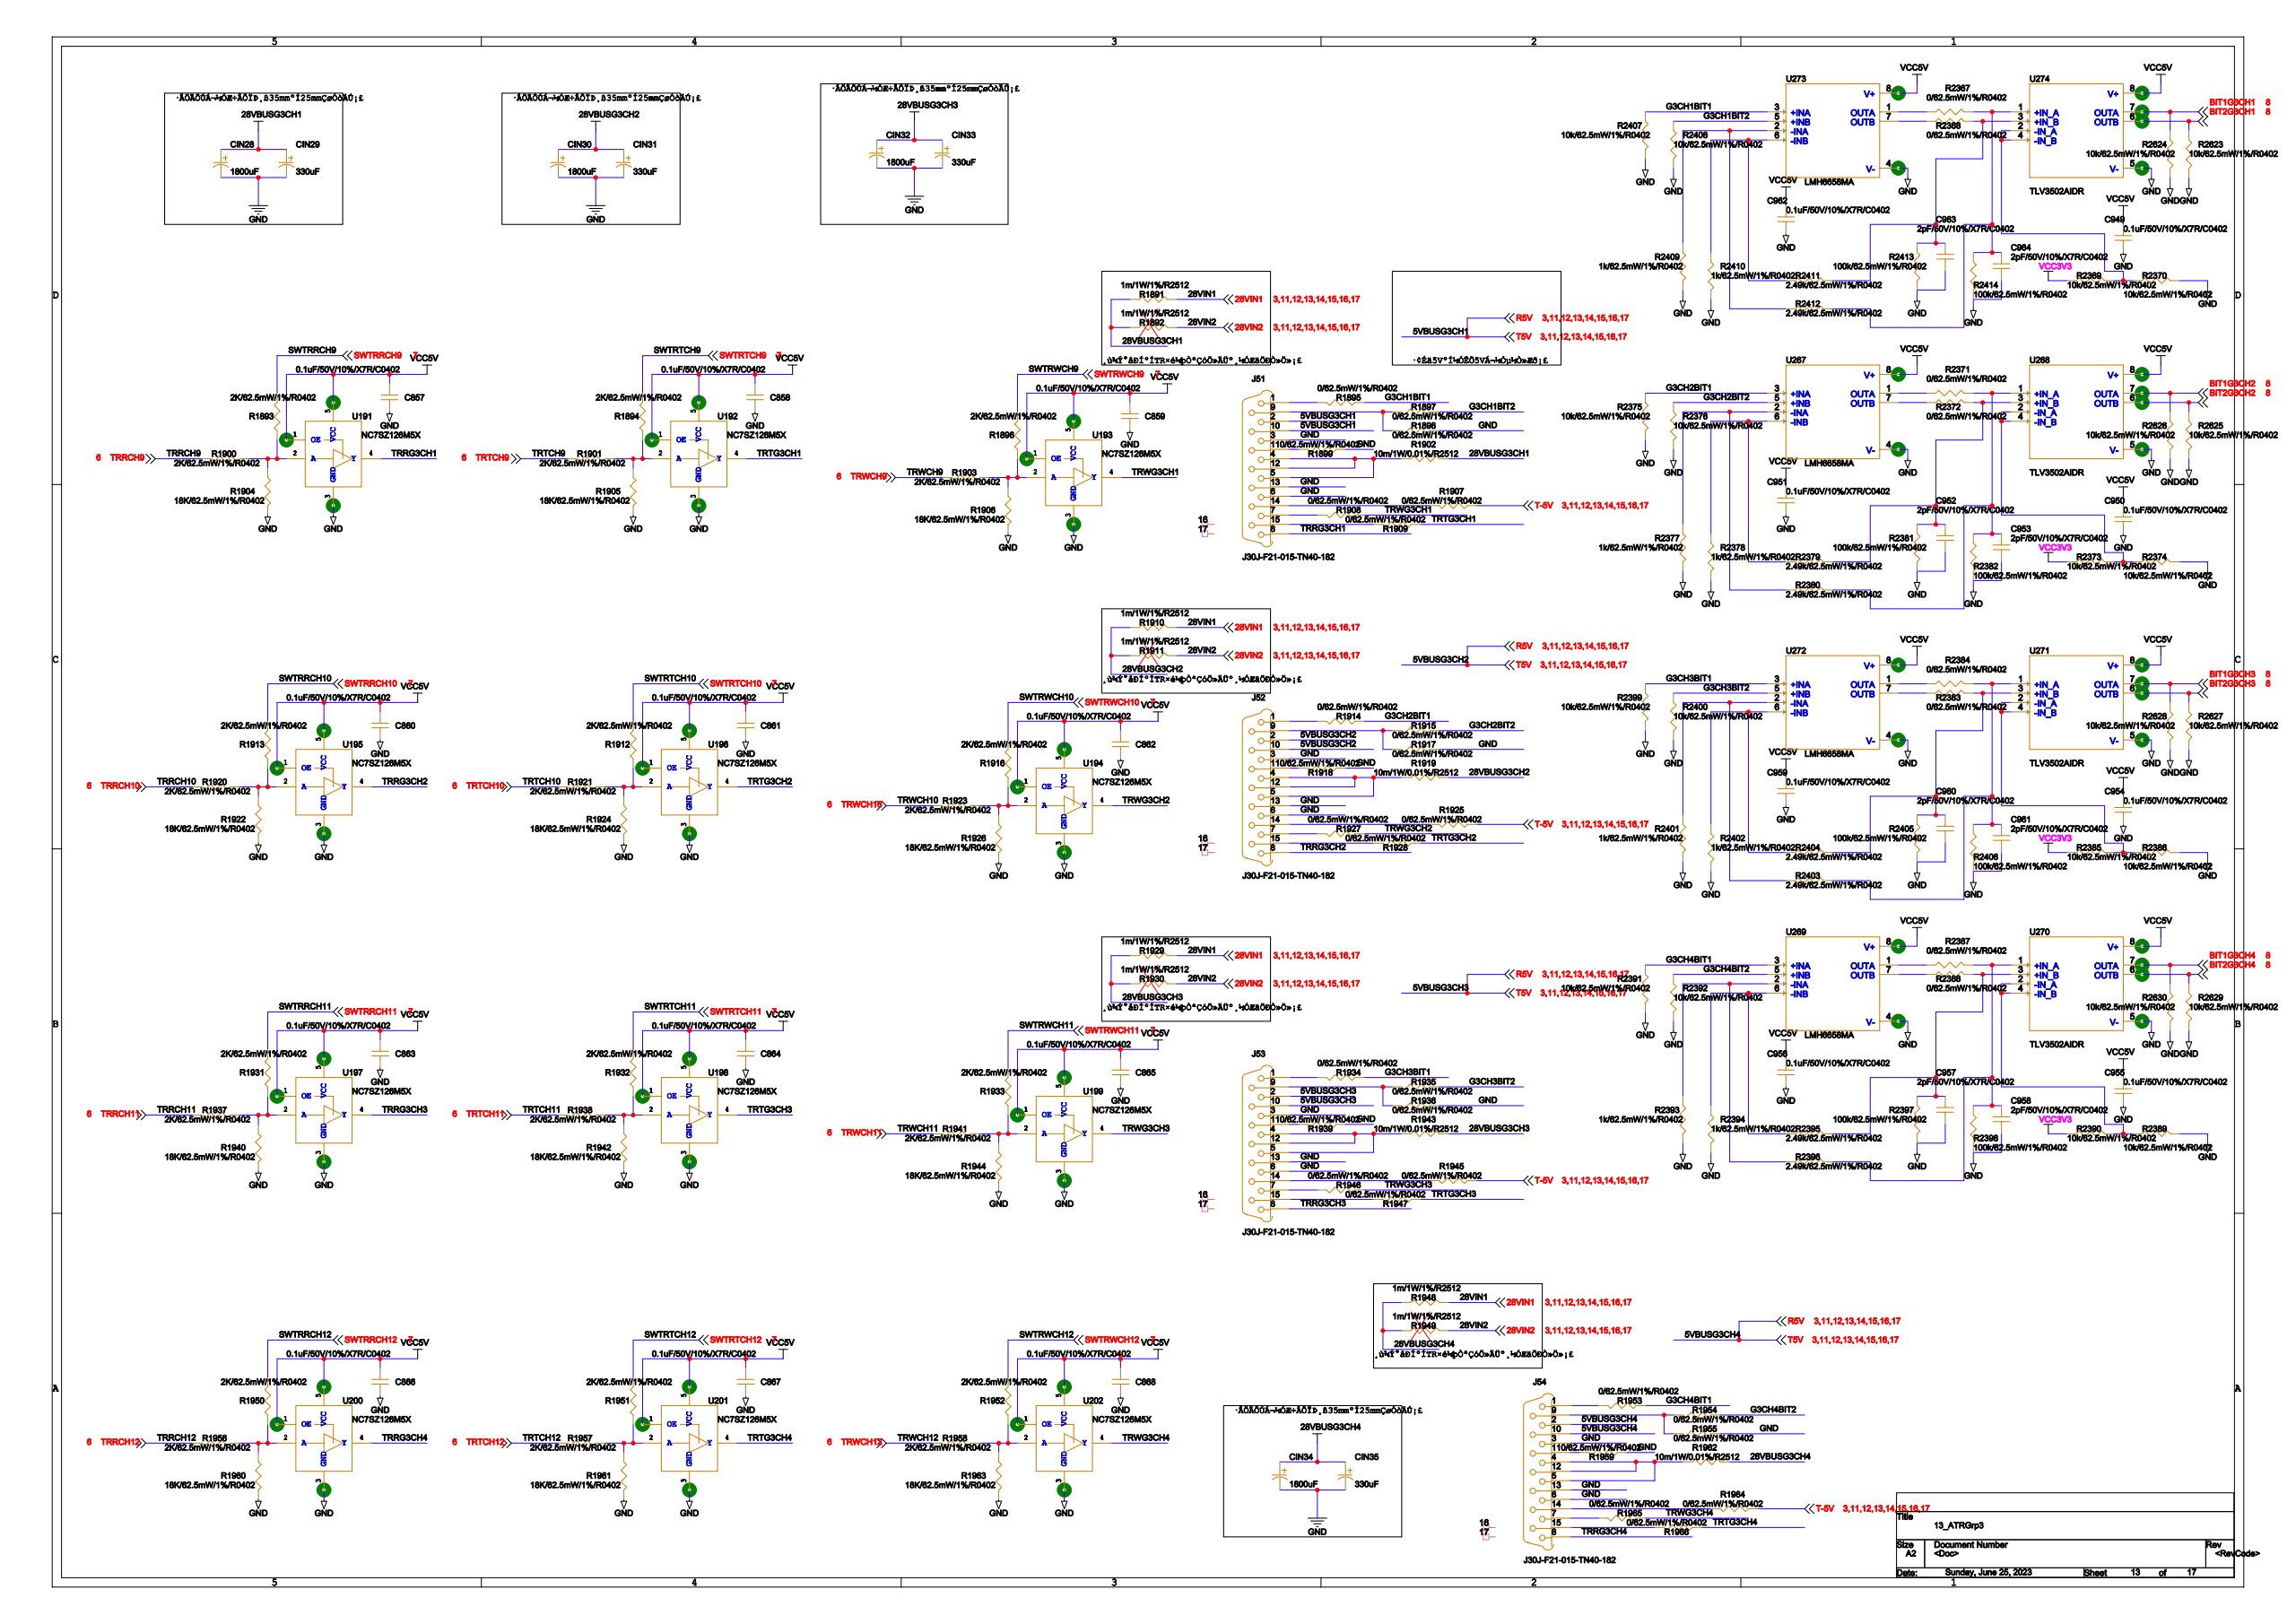Circuit board | Cadence Allegro | 2002 parts | 1538 nets | one sheet of the schematic
Parts on this sheet (reference | value | footprint):
C857 | 0.1uF/50V/10%/X7R/C0402 | 0402
C858 | 0.1uF/50V/10%/X7R/C0402 | 0402
C859 | 0.1uF/50V/10%/X7R/C0402 | 0402
C860 | 0.1uF/50V/10%/X7R/C0402 | 0402
C861 | 0.1uF/50V/10%/X7R/C0402 | 0402
C862 | 0.1uF/50V/10%/X7R/C0402 | 0402
C863 | 0.1uF/50V/10%/X7R/C0402 | 0402
C864 | 0.1uF/50V/10%/X7R/C0402 | 0402
C865 | 0.1uF/50V/10%/X7R/C0402 | 0402
C866 | 0.1uF/50V/10%/X7R/C0402 | 0402
C867 | 0.1uF/50V/10%/X7R/C0402 | 0402
C868 | 0.1uF/50V/10%/X7R/C0402 | 0402
C949 | 0.1uF/50V/10%/X7R/C0402 | 0402
C950 | 0.1uF/50V/10%/X7R/C0402 | 0402
C952 | 2pF/50V/10%/X7R/C0402 | 0402
C953 | 2pF/50V/10%/X7R/C0402 | 0402
C954 | 0.1uF/50V/10%/X7R/C0402 | 0402
C955 | 0.1uF/50V/10%/X7R/C0402 | 0402
C957 | 2pF/50V/10%/X7R/C0402 | 0402
C958 | 2pF/50V/10%/X7R/C0402 | 0402
C960 | 2pF/50V/10%/X7R/C0402 | 0402
C961 | 2pF/50V/10%/X7R/C0402 | 0402
C963 | 2pF/50V/10%/X7R/C0402 | 0402
C964 | 2pF/50V/10%/X7R/C0402 | 0402
CIN28 | ECF1HM182M27OTPO | AP-SMD_BD18-L27-W6_6-LS7_21
CIN29 | ECF1JM331G20OTPO | AP-SMD_BD10-L20-W6_6-LS7_21
CIN30 | ECF1HM182M27OTPO | AP-SMD_BD18-L27-W6_6-LS7_21
CIN31 | ECF1JM331G20OTPO | AP-SMD_BD10-L20-W6_6-LS7_21
CIN32 | ECF1HM182M27OTPO | AP-SMD_BD18-L27-W6_6-LS7_21
CIN33 | ECF1JM331G20OTPO | AP-SMD_BD10-L20-W6_6-LS7_21
CIN34 | ECF1HM182M27OTPO | AP-SMD_BD18-L27-W6_6-LS7_21
CIN35 | ECF1JM331G20OTPO | AP-SMD_BD10-L20-W6_6-LS7_21
J51 | J30J-F21-015-TN40-182 | J30J-F21-015-TN40-182
J52 | J30J-F21-015-TN40-182 | J30J-F21-015-TN40-182
J53 | J30J-F21-015-TN40-182 | J30J-F21-015-TN40-182
J54 | J30J-F21-015-TN40-182 | J30J-F21-015-TN40-182
R1891 | 1m/1W/1%/R2512 | 2512
R1892 | 1m/1W/1%/R2512 | 2512
R1893 | 2K/62.5mW/1%/R0402 | 0402
R1894 | 2K/62.5mW/1%/R0402 | 0402
R1895 | 0/62.5mW/1%/R0402 | 0402
R1896 | 2K/62.5mW/1%/R0402 | 0402
R1897 | 0/62.5mW/1%/R0402 | 0402
R1898 | 0/62.5mW/1%/R0402 | 0402
R1899 | 0/62.5mW/1%/R0402 | 0402
R1900 | 2K/62.5mW/1%/R0402 | 0402
R1901 | 2K/62.5mW/1%/R0402 | 0402
R1902 | 10m/1W/0.01%/R2512 | 2512
R1903 | 2K/62.5mW/1%/R0402 | 0402
R1904 | 18K/62.5mW/1%/R0402 | 0402
R1905 | 18K/62.5mW/1%/R0402 | 0402
R1906 | 18K/62.5mW/1%/R0402 | 0402
R1907 | 0/62.5mW/1%/R0402 | 0402
R1908 | 0/62.5mW/1%/R0402 | 0402
R1909 | 0/62.5mW/1%/R0402 | 0402
R1910 | 1m/1W/1%/R2512 | 2512
R1911 | 1m/1W/1%/R2512 | 2512
R1912 | 2K/62.5mW/1%/R0402 | 0402
R1913 | 2K/62.5mW/1%/R0402 | 0402
R1914 | 0/62.5mW/1%/R0402 | 0402
R1915 | 0/62.5mW/1%/R0402 | 0402
R1916 | 2K/62.5mW/1%/R0402 | 0402
R1917 | 0/62.5mW/1%/R0402 | 0402
R1918 | 0/62.5mW/1%/R0402 | 0402
R1919 | 10m/1W/0.01%/R2512 | 2512
R1920 | 2K/62.5mW/1%/R0402 | 0402
R1921 | 2K/62.5mW/1%/R0402 | 0402
R1922 | 18K/62.5mW/1%/R0402 | 0402
R1923 | 2K/62.5mW/1%/R0402 | 0402
R1924 | 18K/62.5mW/1%/R0402 | 0402
R1925 | 0/62.5mW/1%/R0402 | 0402
R1926 | 18K/62.5mW/1%/R0402 | 0402
R1927 | 0/62.5mW/1%/R0402 | 0402
R1928 | 0/62.5mW/1%/R0402 | 0402
R1929 | 1m/1W/1%/R2512 | 2512
R1930 | 1m/1W/1%/R2512 | 2512
R1931 | 2K/62.5mW/1%/R0402 | 0402
R1932 | 2K/62.5mW/1%/R0402 | 0402
R1933 | 2K/62.5mW/1%/R0402 | 0402
R1934 | 0/62.5mW/1%/R0402 | 0402
R1935 | 0/62.5mW/1%/R0402 | 0402
R1936 | 0/62.5mW/1%/R0402 | 0402
R1937 | 2K/62.5mW/1%/R0402 | 0402
R1938 | 2K/62.5mW/1%/R0402 | 0402
R1939 | 0/62.5mW/1%/R0402 | 0402
R1940 | 18K/62.5mW/1%/R0402 | 0402
R1941 | 2K/62.5mW/1%/R0402 | 0402
R1942 | 18K/62.5mW/1%/R0402 | 0402
R1943 | 10m/1W/0.01%/R2512 | 2512
R1944 | 18K/62.5mW/1%/R0402 | 0402
R1945 | 0/62.5mW/1%/R0402 | 0402
R1946 | 0/62.5mW/1%/R0402 | 0402
R1947 | 0/62.5mW/1%/R0402 | 0402
R1948 | 1m/1W/1%/R2512 | 2512
R1949 | 1m/1W/1%/R2512 | 2512
R1950 | 2K/62.5mW/1%/R0402 | 0402
R1951 | 2K/62.5mW/1%/R0402 | 0402
R1952 | 2K/62.5mW/1%/R0402 | 0402
R1953 | 0/62.5mW/1%/R0402 | 0402
R1954 | 0/62.5mW/1%/R0402 | 0402
R1955 | 0/62.5mW/1%/R0402 | 0402
R1956 | 2K/62.5mW/1%/R0402 | 0402
R1957 | 2K/62.5mW/1%/R0402 | 0402
R1958 | 2K/62.5mW/1%/R0402 | 0402
R1959 | 0/62.5mW/1%/R0402 | 0402
R1960 | 18K/62.5mW/1%/R0402 | 0402
R1961 | 18K/62.5mW/1%/R0402 | 0402
R1962 | 10m/1W/0.01%/R2512 | 2512
R1963 | 18K/62.5mW/1%/R0402 | 0402
R1964 | 0/62.5mW/1%/R0402 | 0402
R1965 | 0/62.5mW/1%/R0402 | 0402
R1966 | 0/62.5mW/1%/R0402 | 0402
R2367 | 0/62.5mW/1%/R0402 | 0402
R2368 | 0/62.5mW/1%/R0402 | 0402
R2369 | 10k/62.5mW/1%/R0402 | 0402
R2370 | 10k/62.5mW/1%/R0402 | 0402
R2371 | 0/62.5mW/1%/R0402 | 0402
R2372 | 0/62.5mW/1%/R0402 | 0402
R2373 | 10k/62.5mW/1%/R0402 | 0402
R2374 | 10k/62.5mW/1%/R0402 | 0402
R2375 | 10k/62.5mW/1%/R0402 | 0402
R2376 | 10k/62.5mW/1%/R0402 | 0402
R2377 | 1K/62.5mW/1%/R0402 | 0402
R2378 | 1K/62.5mW/1%/R0402 | 0402
R2380 | 2.49k/62.5mW/1%/R0402 | 0402
R2381 | 100k/62.5mW/1%/R0402 | 0402
R2382 | 100k/62.5mW/1%/R0402 | 0402
R2383 | 0/62.5mW/1%/R0402 | 0402
R2384 | 0/62.5mW/1%/R0402 | 0402
R2385 | 10k/62.5mW/1%/R0402 | 0402
R2386 | 10k/62.5mW/1%/R0402 | 0402
R2387 | 0/62.5mW/1%/R0402 | 0402
R2388 | 0/62.5mW/1%/R0402 | 0402
R2389 | 10k/62.5mW/1%/R0402 | 0402
R2390 | 10k/62.5mW/1%/R0402 | 0402
R2391 | 10k/62.5mW/1%/R0402 | 0402
R2392 | 10k/62.5mW/1%/R0402 | 0402
R2393 | 1K/62.5mW/1%/R0402 | 0402
R2394 | 1K/62.5mW/1%/R0402 | 0402
R2396 | 2.49k/62.5mW/1%/R0402 | 0402
R2397 | 100k/62.5mW/1%/R0402 | 0402
R2398 | 100k/62.5mW/1%/R0402 | 0402
R2399 | 10k/62.5mW/1%/R0402 | 0402
R2400 | 10k/62.5mW/1%/R0402 | 0402
R2401 | 1K/62.5mW/1%/R0402 | 0402
R2402 | 1K/62.5mW/1%/R0402 | 0402
R2403 | 2.49k/62.5mW/1%/R0402 | 0402
R2404 | 2.49k/62.5mW/1%/R0402 | 0402
R2405 | 100k/62.5mW/1%/R0402 | 0402
R2406 | 100k/62.5mW/1%/R0402 | 0402
R2407 | 10k/62.5mW/1%/R0402 | 0402
R2408 | 10k/62.5mW/1%/R0402 | 0402
R2409 | 1K/62.5mW/1%/R0402 | 0402
R2410 | 1K/62.5mW/1%/R0402 | 0402
R2412 | 2.49k/62.5mW/1%/R0402 | 0402
R2413 | 100k/62.5mW/1%/R0402 | 0402
R2414 | 100k/62.5mW/1%/R0402 | 0402
R2623 | 10k/62.5mW/1%/R0402 | 0402
R2624 | 10k/62.5mW/1%/R0402 | 0402
R2625 | 10k/62.5mW/1%/R0402 | 0402
R2626 | 10k/62.5mW/1%/R0402 | 0402
R2627 | 10k/62.5mW/1%/R0402 | 0402
R2628 | 10k/62.5mW/1%/R0402 | 0402
R2629 | 10k/62.5mW/1%/R0402 | 0402
R2630 | 10k/62.5mW/1%/R0402 | 0402
U191 | NC7SZ126M5X | SOT-23-5
U192 | NC7SZ126M5X | SOT-23-5
U193 | NC7SZ126M5X | SOT-23-5
U194 | NC7SZ126M5X | SOT-23-5
U195 | NC7SZ126M5X | SOT-23-5
U196 | NC7SZ126M5X | SOT-23-5
U197 | NC7SZ126M5X | SOT-23-5
U198 | NC7SZ126M5X | SOT-23-5
U199 | NC7SZ126M5X | SOT-23-5
U200 | NC7SZ126M5X | SOT-23-5
U201 | NC7SZ126M5X | SOT-23-5
U202 | NC7SZ126M5X | SOT-23-5
U267 | LMH6658MA | SOIC127P599X175-8N
U269 | LMH6658MA | SOIC127P599X175-8N
U271 | TLV3502AIDR | SOIC127P599X175-8N
U273 | LMH6658MA | SOIC127P599X175-8N
Nets of these parts (net: part-pin ...):
3.3V: R2369-1 R2373-1 R2385-1 R2390-1
AGND: C857-2 C858-2 C859-2 C860-2 C861-2 C862-2 C863-2 C864-2 C865-2 C866-2 C867-2 C868-2 C949-2 C950-2 C952-2 C953-2 C954-2 C955-2 C957-2 C958-2 C960-2 C961-2 C963-2 C964-2 CIN28-2 CIN29-2 CIN30-2 CIN31-2 CIN32-2 CIN33-2 CIN34-2 CIN35-2 J51-3 J51-6 J51-13 J52-3 J52-6 J52-13 J53-3 J53-6 J53-13 J54-3 J54-6 J54-13 R1898-1 R1899-1 R1904-1 R1905-1 R1906-1 R1917-1 R1918-1 R1922-1 R1924-1 R1926-1 R1936-1 R1939-1 R1940-1 R1942-1 R1944-1 R1955-1 R1959-1 R1960-1 R1961-1 R1963-1 R2370-2 R2374-2 R2375-2 R2376-2 R2377-2 R2378-2 R2381-2 R2382-2 R2386-2 R2389-2 R2391-2 R2392-2 R2393-2 R2394-2 R2397-2 R2398-2 R2399-2 R2400-2 R2401-2 R2402-2 R2405-2 R2406-2 R2407-2 R2408-2 R2409-2 R2410-2 R2413-2 R2414-2 R2623-2 R2624-2 R2625-2 R2626-2 R2627-2 R2628-2 R2629-2 R2630-2 U191-3 U192-3 U193-3 U194-3 U195-3 U196-3 U197-3 U198-3 U199-3 U200-3 U201-3 U202-3 U267-4 U269-4 U271-5 U273-4
VCC5V: C857-1 C858-1 C859-1 C860-1 C861-1 C862-1 C863-1 C864-1 C865-1 C866-1 C867-1 C868-1 C949-1 C950-1 C954-1 C955-1 U191-1 U191-5 U192-1 U192-5 U193-1 U193-5 U194-1 U194-5 U195-1 U195-5 U196-1 U196-5 U197-1 U197-5 U198-1 U198-5 U199-1 U199-5 U200-1 U200-5 U201-1 U201-5 U202-1 U202-5 U267-8 U269-8 U271-8 U273-8
28VIN1: R1891-2 R1892-2 R1910-2 R1911-2 R1929-2 R1930-2 R1948-2 R1949-2
R5V: J51-2 J51-10 J52-2 J52-10 J53-2 J53-10 J54-2 J54-10
T-5V: R1907-1 R1925-1 R1945-1 R1964-1
N24399384: R2378-1 U267-6
N24399394: C952-1 R2372-2 R2381-1
N24399372: R2377-1 R2380-1 U267-2
N24399392: C953-1 R2371-2 R2380-2 R2382-1
N24399938: R2394-1 U269-6
N24399948: C957-1 R2388-2 R2397-1
N24399926: R2393-1 R2396-1 U269-2
N24399946: C958-1 R2387-2 R2396-2 R2398-1
N24399750: R2401-1 R2403-1
N24399766: C961-1 R2384-2 R2403-2 R2406-1 U271-1
N24399754: R2402-1 R2404-1
N24399768: C960-1 R2383-2 R2404-2 R2405-1 U271-3
N24399204: R2410-1 U273-6
N24399214: C963-1 R2368-2 R2413-1
N24399200: R2409-1 R2412-1 U273-2
N24399212: C964-1 R2367-2 R2412-2 R2414-1
G3CH2BIT1: R1914-1 R2375-1 U267-3
G3CH2BIT2: R1915-1 R2376-1 U267-5
N24399388: R2371-1 U267-1
N24399390: R2372-1 U267-7
G3CH4BIT1: R1953-1 R2391-1 U269-3
G3CH4BIT2: R1954-1 R2392-1 U269-5
N24399942: R2387-1 U269-1
N24399944: R2388-1 U269-7
G3CH3BIT1: R1934-1 R2399-1
G3CH3BIT2: R1935-1 R2400-1
N24399762: R2384-1
N24399764: R2383-1
G3CH1BIT1: R1895-1 R2407-1 U273-3
G3CH1BIT2: R1897-1 R2408-1 U273-5
N24399208: R2367-1 U273-1
N24399210: R2368-1 U273-7
N24399446: R2373-2 R2374-1
BIT1G3CH2: R2626-1
BIT2G3CH2: R2625-1
N24400000: R2389-1 R2390-2
BIT1G3CH4: R2630-1
BIT2G3CH4: R2629-1
N24399820: R2385-2 R2386-1 U271-2 U271-4
BIT1G3CH3: R2628-1 U271-7
BIT2G3CH3: R2627-1 U271-6
N24399266: R2369-2 R2370-1
BIT1G3CH1: R2624-1
BIT2G3CH1: R2623-1
N23725346: J51-1 R1895-2
N23725359: J51-11 R1899-2
N23725361: J51-4 J51-5 J51-12 R1902-1
N23725373: J51-14 R1907-2
N23725377: J51-15 R1909-2
N23725375: J51-7 R1908-2
TRRG3CH1: J51-8 U191-4
N23725348: J51-9 R1897-2 R1898-2
N23725905: J52-1 R1914-2
N23725918: J52-11 R1918-2
N23725920: J52-4 J52-5 J52-12 R1919-1
N23725932: J52-14 R1925-2
N23725936: J52-15 R1928-2
N23725934: J52-7 R1927-2
TRRG3CH2: J52-8 U195-4
N23725907: J52-9 R1915-2 R1917-2
N23726532: J53-1 R1934-2
N23726545: J53-11 R1939-2
N23726547: J53-4 J53-5 J53-12 R1943-1
N23726559: J53-14 R1945-2
N23726563: J53-15 R1947-2
N23726561: J53-7 R1946-2
TRRG3CH3: J53-8 U197-4
N23726534: J53-9 R1935-2 R1936-2
N23727336: J54-1 R1953-2
N23727349: J54-11 R1959-2
N23727351: J54-4 J54-5 J54-12 R1962-1
N23727363: J54-14 R1964-2
N23727367: J54-15 R1966-2
N23727365: J54-7 R1965-2
TRRG3CH4: J54-8 U200-4
N23727338: J54-9 R1954-2 R1955-2
28VBUSG3CH1: CIN28-1 CIN29-1 R1891-1 R1892-1 R1902-2
28VBUSG3CH2: CIN30-1 CIN31-1 R1910-1 R1911-1 R1919-2
28VBUSG3CH3: CIN32-1 CIN33-1 R1929-1 R1930-1 R1943-2
28VBUSG3CH4: CIN34-1 CIN35-1 R1948-1 R1949-1 R1962-2
SWTRRCH9: R1893-1
N24007480: R1893-2 R1900-2 R1904-2 U191-2
SWTRTCH9: R1894-1
N24006500: R1894-2 R1901-2 R1905-2 U192-2
SWTRWCH9: R1896-1
N24006988: R1896-2 R1903-2 R1906-2 U193-2
TRRCH9: R1900-1
TRTCH9: R1901-1
TRWCH9: R1903-1
SWTRTCH10: R1912-1
N24006618: R1912-2 R1921-2 R1924-2 U196-2
SWTRRCH10: R1913-1
N24007598: R1913-2 R1920-2 R1922-2 U195-2
SWTRWCH10: R1916-1
N24007110: R1916-2 R1923-2 R1926-2 U194-2
TRRCH10: R1920-1
TRTCH10: R1921-1
TRWCH10: R1923-1
SWTRRCH11: R1931-1
N24007724: R1931-2 R1937-2 R1940-2 U197-2
SWTRTCH11: R1932-1
N24006744: R1932-2 R1938-2 R1942-2 U198-2
SWTRWCH11: R1933-1
N24007232: R1933-2 R1941-2 R1944-2 U199-2
TRRCH11: R1937-1
TRTCH11: R1938-1
TRWCH11: R1941-1
SWTRRCH12: R1950-1
N24007842: R1950-2 R1956-2 R1960-2 U200-2
SWTRTCH12: R1951-1
N24006866: R1951-2 R1957-2 R1961-2 U201-2
SWTRWCH12: R1952-1
N24007354: R1952-2 R1958-2 R1963-2 U202-2
TRRCH12: R1956-1
TRTCH12: R1957-1
TRWCH12: R1958-1
TRTG3CH1: R1909-1 U192-4
TRWG3CH1: R1908-1 U193-4
TRWG3CH2: R1927-1 U194-4
TRTG3CH2: R1928-1 U196-4
TRTG3CH3: R1947-1 U198-4
TRWG3CH3: R1946-1 U199-4
TRTG3CH4: R1966-1 U201-4
TRWG3CH4: R1965-1 U202-4